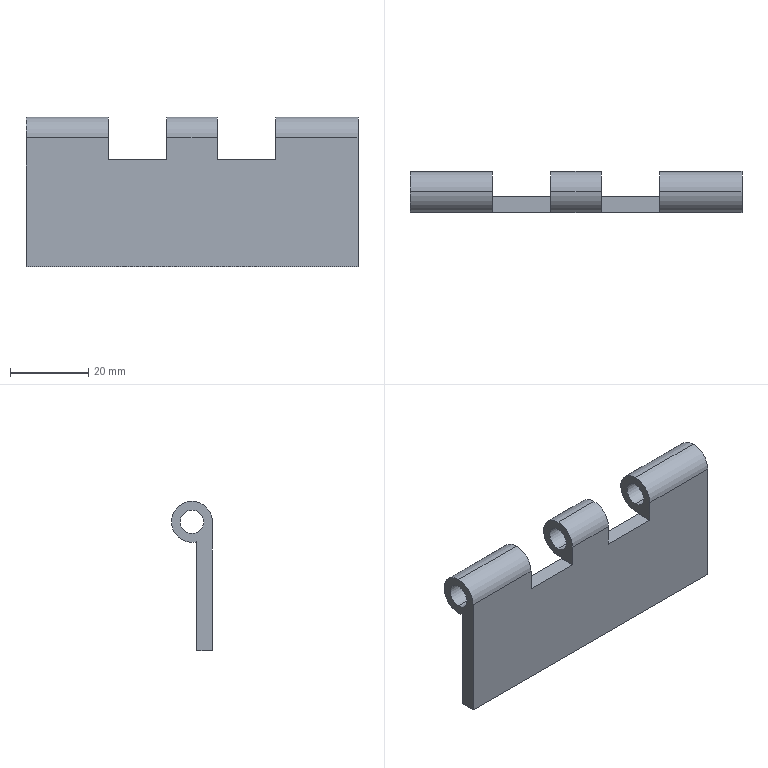Part | SolidWorks | features ICE 2, Chamfer 1, Cut 1, Extrusion 1 | 1 solid | 26 faces | box 85 x 10.5 x 38.25 mm | volume 12934 mm3 | cylinder 15 | plane 11 | commonest cylinder face diameters 10.5 x9 6 x6
STEP:
#1=CARTESIAN_POINT('',(21.5,0.,3.));
#2=VERTEX_POINT('',#1);
#3=CARTESIAN_POINT('',(21.5,0.,-3.));
#4=VERTEX_POINT('',#3);
#5=CARTESIAN_POINT('',(21.5,0.,0.));
#6=DIRECTION('',(1.,0.,0.));
#7=DIRECTION('',(0.,0.,-1.));
#8=AXIS2_PLACEMENT_3D('',#5,#6,#7);
#9=CIRCLE('',#8,3.);
#10=EDGE_CURVE('',#2,#4,#9,.T.);
#11=ORIENTED_EDGE('',*,*,#10,.F.);
#12=CARTESIAN_POINT('',(42.5,0.,3.));
#13=VERTEX_POINT('',#12);
#14=CARTESIAN_POINT('',(-42.5,0.,3.));
#15=DIRECTION('',(1.,0.,0.));
#16=VECTOR('',#15,1000.);
#17=LINE('',#14,#16);
#18=EDGE_CURVE('',#2,#13,#17,.T.);
#19=ORIENTED_EDGE('',*,*,#18,.T.);
#20=CARTESIAN_POINT('',(42.5,0.,-3.));
#21=VERTEX_POINT('',#20);
#22=CARTESIAN_POINT('',(42.5,0.,0.));
#23=DIRECTION('',(1.,0.,0.));
#24=DIRECTION('',(0.,0.,-1.));
#25=AXIS2_PLACEMENT_3D('',#22,#23,#24);
#26=CIRCLE('',#25,3.);
#27=EDGE_CURVE('',#13,#21,#26,.T.);
#28=ORIENTED_EDGE('',*,*,#27,.T.);
#29=CARTESIAN_POINT('',(-42.5,0.,-3.));
#30=DIRECTION('',(1.,0.,0.));
#31=VECTOR('',#30,1000.);
#32=LINE('',#29,#31);
#33=EDGE_CURVE('',#4,#21,#32,.T.);
#34=ORIENTED_EDGE('',*,*,#33,.F.);
#35=EDGE_LOOP('',(#11,#19,#28,#34));
#36=FACE_OUTER_BOUND('',#35,.T.);
#37=CARTESIAN_POINT('',(-42.5,0.,0.));
#38=DIRECTION('',(1.,0.,0.));
#39=DIRECTION('',(0.,0.,-1.));
#40=AXIS2_PLACEMENT_3D('',#37,#38,#39);
#41=CYLINDRICAL_SURFACE('',#40,3.);
#42=ADVANCED_FACE('',(#36),#41,.F.);
#43=CARTESIAN_POINT('',(-6.5,0.,3.));
#44=VERTEX_POINT('',#43);
#45=CARTESIAN_POINT('',(-6.5,0.,-3.));
#46=VERTEX_POINT('',#45);
#47=CARTESIAN_POINT('',(-6.5,0.,0.));
#48=DIRECTION('',(1.,0.,0.));
#49=DIRECTION('',(0.,0.,-1.));
#50=AXIS2_PLACEMENT_3D('',#47,#48,#49);
#51=CIRCLE('',#50,3.);
#52=EDGE_CURVE('',#44,#46,#51,.T.);
#53=ORIENTED_EDGE('',*,*,#52,.F.);
#54=CARTESIAN_POINT('',(6.5,0.,3.));
#55=VERTEX_POINT('',#54);
#56=CARTESIAN_POINT('',(-42.5,0.,3.));
#57=DIRECTION('',(1.,0.,0.));
#58=VECTOR('',#57,1000.);
#59=LINE('',#56,#58);
#60=EDGE_CURVE('',#44,#55,#59,.T.);
#61=ORIENTED_EDGE('',*,*,#60,.T.);
#62=CARTESIAN_POINT('',(6.5,0.,-3.));
#63=VERTEX_POINT('',#62);
#64=CARTESIAN_POINT('',(6.5,0.,0.));
#65=DIRECTION('',(-1.,0.,0.));
#66=DIRECTION('',(0.,0.,1.));
#67=AXIS2_PLACEMENT_3D('',#64,#65,#66);
#68=CIRCLE('',#67,3.);
#69=EDGE_CURVE('',#63,#55,#68,.T.);
#70=ORIENTED_EDGE('',*,*,#69,.F.);
#71=CARTESIAN_POINT('',(-42.5,0.,-3.));
#72=DIRECTION('',(1.,0.,0.));
#73=VECTOR('',#72,1000.);
#74=LINE('',#71,#73);
#75=EDGE_CURVE('',#46,#63,#74,.T.);
#76=ORIENTED_EDGE('',*,*,#75,.F.);
#77=EDGE_LOOP('',(#53,#61,#70,#76));
#78=FACE_OUTER_BOUND('',#77,.T.);
#79=CARTESIAN_POINT('',(-42.5,0.,0.));
#80=DIRECTION('',(1.,0.,0.));
#81=DIRECTION('',(0.,0.,-1.));
#82=AXIS2_PLACEMENT_3D('',#79,#80,#81);
#83=CYLINDRICAL_SURFACE('',#82,3.);
#84=ADVANCED_FACE('',(#78),#83,.F.);
#85=CARTESIAN_POINT('',(-42.5,0.,3.));
#86=VERTEX_POINT('',#85);
#87=CARTESIAN_POINT('',(-42.5,0.,-3.));
#88=VERTEX_POINT('',#87);
#89=CARTESIAN_POINT('',(-42.5,0.,0.));
#90=DIRECTION('',(1.,0.,0.));
#91=DIRECTION('',(0.,0.,-1.));
#92=AXIS2_PLACEMENT_3D('',#89,#90,#91);
#93=CIRCLE('',#92,3.);
#94=EDGE_CURVE('',#86,#88,#93,.T.);
#95=ORIENTED_EDGE('',*,*,#94,.F.);
#96=CARTESIAN_POINT('',(-21.5,0.,3.));
#97=VERTEX_POINT('',#96);
#98=CARTESIAN_POINT('',(-42.5,0.,3.));
#99=DIRECTION('',(1.,0.,0.));
#100=VECTOR('',#99,1000.);
#101=LINE('',#98,#100);
#102=EDGE_CURVE('',#86,#97,#101,.T.);
#103=ORIENTED_EDGE('',*,*,#102,.T.);
#104=CARTESIAN_POINT('',(-21.5,0.,-3.));
#105=VERTEX_POINT('',#104);
#106=CARTESIAN_POINT('',(-21.5,0.,0.));
#107=DIRECTION('',(-1.,0.,0.));
#108=DIRECTION('',(0.,0.,1.));
#109=AXIS2_PLACEMENT_3D('',#106,#107,#108);
#110=CIRCLE('',#109,3.);
#111=EDGE_CURVE('',#105,#97,#110,.T.);
#112=ORIENTED_EDGE('',*,*,#111,.F.);
#113=CARTESIAN_POINT('',(-42.5,0.,-3.));
#114=DIRECTION('',(1.,0.,0.));
#115=VECTOR('',#114,1000.);
#116=LINE('',#113,#115);
#117=EDGE_CURVE('',#88,#105,#116,.T.);
#118=ORIENTED_EDGE('',*,*,#117,.F.);
#119=EDGE_LOOP('',(#95,#103,#112,#118));
#120=FACE_OUTER_BOUND('',#119,.T.);
#121=CARTESIAN_POINT('',(-42.5,0.,0.));
#122=DIRECTION('',(1.,0.,0.));
#123=DIRECTION('',(0.,0.,-1.));
#124=AXIS2_PLACEMENT_3D('',#121,#122,#123);
#125=CYLINDRICAL_SURFACE('',#124,3.);
#126=ADVANCED_FACE('',(#120),#125,.F.);
#127=CARTESIAN_POINT('',(-21.5,0.,5.25));
#128=VERTEX_POINT('',#127);
#129=CARTESIAN_POINT('',(-21.5,0.,-5.25));
#130=VERTEX_POINT('',#129);
#131=CARTESIAN_POINT('',(-21.5,0.,0.));
#132=DIRECTION('',(-1.,0.,0.));
#133=DIRECTION('',(0.,0.,1.));
#134=AXIS2_PLACEMENT_3D('',#131,#132,#133);
#135=CIRCLE('',#134,5.25);
#136=EDGE_CURVE('',#128,#130,#135,.T.);
#137=ORIENTED_EDGE('',*,*,#136,.T.);
#138=CARTESIAN_POINT('',(-42.5,0.,-5.25));
#139=VERTEX_POINT('',#138);
#140=CARTESIAN_POINT('',(42.5,0.,-5.25));
#141=DIRECTION('',(-1.,0.,0.));
#142=VECTOR('',#141,1000.);
#143=LINE('',#140,#142);
#144=EDGE_CURVE('',#130,#139,#143,.T.);
#145=ORIENTED_EDGE('',*,*,#144,.T.);
#146=CARTESIAN_POINT('',(-42.5,0.,5.25));
#147=VERTEX_POINT('',#146);
#148=CARTESIAN_POINT('',(-42.5,0.,0.));
#149=DIRECTION('',(1.,0.,0.));
#150=DIRECTION('',(0.,0.,-1.));
#151=AXIS2_PLACEMENT_3D('',#148,#149,#150);
#152=CIRCLE('',#151,5.25);
#153=EDGE_CURVE('',#139,#147,#152,.T.);
#154=ORIENTED_EDGE('',*,*,#153,.T.);
#155=CARTESIAN_POINT('',(42.5,0.,5.25));
#156=DIRECTION('',(-1.,0.,0.));
#157=VECTOR('',#156,1000.);
#158=LINE('',#155,#157);
#159=EDGE_CURVE('',#128,#147,#158,.T.);
#160=ORIENTED_EDGE('',*,*,#159,.F.);
#161=EDGE_LOOP('',(#137,#145,#154,#160));
#162=FACE_OUTER_BOUND('',#161,.T.);
#163=CARTESIAN_POINT('',(42.5,0.,0.));
#164=DIRECTION('',(-1.,0.,0.));
#165=DIRECTION('',(0.,0.,1.));
#166=AXIS2_PLACEMENT_3D('',#163,#164,#165);
#167=CYLINDRICAL_SURFACE('',#166,5.25);
#168=ADVANCED_FACE('',(#162),#167,.T.);
#169=CARTESIAN_POINT('',(-21.5,-5.25,0.));
#170=VERTEX_POINT('',#169);
#171=CARTESIAN_POINT('',(-21.5,0.,0.));
#172=DIRECTION('',(-1.,0.,0.));
#173=DIRECTION('',(0.,0.,1.));
#174=AXIS2_PLACEMENT_3D('',#171,#172,#173);
#175=CIRCLE('',#174,5.25);
#176=EDGE_CURVE('',#170,#128,#175,.T.);
#177=ORIENTED_EDGE('',*,*,#176,.T.);
#178=ORIENTED_EDGE('',*,*,#159,.T.);
#179=CARTESIAN_POINT('',(-42.5,-5.25,0.));
#180=VERTEX_POINT('',#179);
#181=CARTESIAN_POINT('',(-42.5,0.,0.));
#182=DIRECTION('',(1.,0.,0.));
#183=DIRECTION('',(0.,0.,-1.));
#184=AXIS2_PLACEMENT_3D('',#181,#182,#183);
#185=CIRCLE('',#184,5.25);
#186=EDGE_CURVE('',#147,#180,#185,.T.);
#187=ORIENTED_EDGE('',*,*,#186,.T.);
#188=CARTESIAN_POINT('',(42.5,-5.25,0.));
#189=DIRECTION('',(-1.,0.,0.));
#190=VECTOR('',#189,1000.);
#191=LINE('',#188,#190);
#192=EDGE_CURVE('',#170,#180,#191,.T.);
#193=ORIENTED_EDGE('',*,*,#192,.F.);
#194=EDGE_LOOP('',(#177,#178,#187,#193));
#195=FACE_OUTER_BOUND('',#194,.T.);
#196=CARTESIAN_POINT('',(42.5,0.,0.));
#197=DIRECTION('',(-1.,0.,0.));
#198=DIRECTION('',(0.,0.,1.));
#199=AXIS2_PLACEMENT_3D('',#196,#197,#198);
#200=CYLINDRICAL_SURFACE('',#199,5.25);
#201=ADVANCED_FACE('',(#195),#200,.T.);
#202=CARTESIAN_POINT('',(42.5,0.,-5.25));
#203=VERTEX_POINT('',#202);
#204=CARTESIAN_POINT('',(42.5,0.,5.25));
#205=VERTEX_POINT('',#204);
#206=CARTESIAN_POINT('',(42.5,0.,0.));
#207=DIRECTION('',(1.,0.,0.));
#208=DIRECTION('',(0.,0.,-1.));
#209=AXIS2_PLACEMENT_3D('',#206,#207,#208);
#210=CIRCLE('',#209,5.25);
#211=EDGE_CURVE('',#203,#205,#210,.T.);
#212=ORIENTED_EDGE('',*,*,#211,.F.);
#213=CARTESIAN_POINT('',(21.5,0.,-5.25));
#214=VERTEX_POINT('',#213);
#215=CARTESIAN_POINT('',(42.5,0.,-5.25));
#216=DIRECTION('',(-1.,0.,0.));
#217=VECTOR('',#216,1000.);
#218=LINE('',#215,#217);
#219=EDGE_CURVE('',#203,#214,#218,.T.);
#220=ORIENTED_EDGE('',*,*,#219,.T.);
#221=CARTESIAN_POINT('',(21.5,0.,5.25));
#222=VERTEX_POINT('',#221);
#223=CARTESIAN_POINT('',(21.5,0.,0.));
#224=DIRECTION('',(1.,0.,0.));
#225=DIRECTION('',(0.,0.,-1.));
#226=AXIS2_PLACEMENT_3D('',#223,#224,#225);
#227=CIRCLE('',#226,5.25);
#228=EDGE_CURVE('',#214,#222,#227,.T.);
#229=ORIENTED_EDGE('',*,*,#228,.T.);
#230=CARTESIAN_POINT('',(42.5,0.,5.25));
#231=DIRECTION('',(-1.,0.,0.));
#232=VECTOR('',#231,1000.);
#233=LINE('',#230,#232);
#234=EDGE_CURVE('',#205,#222,#233,.T.);
#235=ORIENTED_EDGE('',*,*,#234,.F.);
#236=EDGE_LOOP('',(#212,#220,#229,#235));
#237=FACE_OUTER_BOUND('',#236,.T.);
#238=CARTESIAN_POINT('',(42.5,0.,0.));
#239=DIRECTION('',(-1.,0.,0.));
#240=DIRECTION('',(0.,0.,1.));
#241=AXIS2_PLACEMENT_3D('',#238,#239,#240);
#242=CYLINDRICAL_SURFACE('',#241,5.25);
#243=ADVANCED_FACE('',(#237),#242,.T.);
#244=CARTESIAN_POINT('',(42.5,-5.25,0.));
#245=VERTEX_POINT('',#244);
#246=CARTESIAN_POINT('',(42.5,0.,0.));
#247=DIRECTION('',(1.,0.,0.));
#248=DIRECTION('',(0.,0.,-1.));
#249=AXIS2_PLACEMENT_3D('',#246,#247,#248);
#250=CIRCLE('',#249,5.25);
#251=EDGE_CURVE('',#205,#245,#250,.T.);
#252=ORIENTED_EDGE('',*,*,#251,.F.);
#253=ORIENTED_EDGE('',*,*,#234,.T.);
#254=CARTESIAN_POINT('',(21.5,-5.25,0.));
#255=VERTEX_POINT('',#254);
#256=CARTESIAN_POINT('',(21.5,0.,0.));
#257=DIRECTION('',(1.,0.,0.));
#258=DIRECTION('',(0.,0.,-1.));
#259=AXIS2_PLACEMENT_3D('',#256,#257,#258);
#260=CIRCLE('',#259,5.25);
#261=EDGE_CURVE('',#222,#255,#260,.T.);
#262=ORIENTED_EDGE('',*,*,#261,.T.);
#263=CARTESIAN_POINT('',(42.5,-5.25,0.));
#264=DIRECTION('',(-1.,0.,0.));
#265=VECTOR('',#264,1000.);
#266=LINE('',#263,#265);
#267=EDGE_CURVE('',#245,#255,#266,.T.);
#268=ORIENTED_EDGE('',*,*,#267,.F.);
#269=EDGE_LOOP('',(#252,#253,#262,#268));
#270=FACE_OUTER_BOUND('',#269,.T.);
#271=CARTESIAN_POINT('',(42.5,0.,0.));
#272=DIRECTION('',(-1.,0.,0.));
#273=DIRECTION('',(0.,0.,1.));
#274=AXIS2_PLACEMENT_3D('',#271,#272,#273);
#275=CYLINDRICAL_SURFACE('',#274,5.25);
#276=ADVANCED_FACE('',(#270),#275,.T.);
#277=CARTESIAN_POINT('',(6.5,0.,5.25));
#278=VERTEX_POINT('',#277);
#279=CARTESIAN_POINT('',(6.5,0.,-5.25));
#280=VERTEX_POINT('',#279);
#281=CARTESIAN_POINT('',(6.5,0.,0.));
#282=DIRECTION('',(-1.,0.,0.));
#283=DIRECTION('',(0.,0.,1.));
#284=AXIS2_PLACEMENT_3D('',#281,#282,#283);
#285=CIRCLE('',#284,5.25);
#286=EDGE_CURVE('',#278,#280,#285,.T.);
#287=ORIENTED_EDGE('',*,*,#286,.T.);
#288=CARTESIAN_POINT('',(-6.5,0.,-5.25));
#289=VERTEX_POINT('',#288);
#290=CARTESIAN_POINT('',(42.5,0.,-5.25));
#291=DIRECTION('',(-1.,0.,0.));
#292=VECTOR('',#291,1000.);
#293=LINE('',#290,#292);
#294=EDGE_CURVE('',#280,#289,#293,.T.);
#295=ORIENTED_EDGE('',*,*,#294,.T.);
#296=CARTESIAN_POINT('',(-6.5,0.,5.25));
#297=VERTEX_POINT('',#296);
#298=CARTESIAN_POINT('',(-6.5,0.,0.));
#299=DIRECTION('',(1.,0.,0.));
#300=DIRECTION('',(0.,0.,-1.));
#301=AXIS2_PLACEMENT_3D('',#298,#299,#300);
#302=CIRCLE('',#301,5.25);
#303=EDGE_CURVE('',#289,#297,#302,.T.);
#304=ORIENTED_EDGE('',*,*,#303,.T.);
#305=CARTESIAN_POINT('',(42.5,0.,5.25));
#306=DIRECTION('',(-1.,0.,0.));
#307=VECTOR('',#306,1000.);
#308=LINE('',#305,#307);
#309=EDGE_CURVE('',#278,#297,#308,.T.);
#310=ORIENTED_EDGE('',*,*,#309,.F.);
#311=EDGE_LOOP('',(#287,#295,#304,#310));
#312=FACE_OUTER_BOUND('',#311,.T.);
#313=CARTESIAN_POINT('',(42.5,0.,0.));
#314=DIRECTION('',(-1.,0.,0.));
#315=DIRECTION('',(0.,0.,1.));
#316=AXIS2_PLACEMENT_3D('',#313,#314,#315);
#317=CYLINDRICAL_SURFACE('',#316,5.25);
#318=ADVANCED_FACE('',(#312),#317,.T.);
#319=CARTESIAN_POINT('',(6.5,-5.25,0.));
#320=VERTEX_POINT('',#319);
#321=CARTESIAN_POINT('',(6.5,0.,0.));
#322=DIRECTION('',(-1.,0.,0.));
#323=DIRECTION('',(0.,0.,1.));
#324=AXIS2_PLACEMENT_3D('',#321,#322,#323);
#325=CIRCLE('',#324,5.25);
#326=EDGE_CURVE('',#320,#278,#325,.T.);
#327=ORIENTED_EDGE('',*,*,#326,.T.);
#328=ORIENTED_EDGE('',*,*,#309,.T.);
#329=CARTESIAN_POINT('',(-6.5,-5.25,0.));
#330=VERTEX_POINT('',#329);
#331=CARTESIAN_POINT('',(-6.5,0.,0.));
#332=DIRECTION('',(1.,0.,0.));
#333=DIRECTION('',(0.,0.,-1.));
#334=AXIS2_PLACEMENT_3D('',#331,#332,#333);
#335=CIRCLE('',#334,5.25);
#336=EDGE_CURVE('',#297,#330,#335,.T.);
#337=ORIENTED_EDGE('',*,*,#336,.T.);
#338=CARTESIAN_POINT('',(42.5,-5.25,0.));
#339=DIRECTION('',(-1.,0.,0.));
#340=VECTOR('',#339,1000.);
#341=LINE('',#338,#340);
#342=EDGE_CURVE('',#320,#330,#341,.T.);
#343=ORIENTED_EDGE('',*,*,#342,.F.);
#344=EDGE_LOOP('',(#327,#328,#337,#343));
#345=FACE_OUTER_BOUND('',#344,.T.);
#346=CARTESIAN_POINT('',(42.5,0.,0.));
#347=DIRECTION('',(-1.,0.,0.));
#348=DIRECTION('',(0.,0.,1.));
#349=AXIS2_PLACEMENT_3D('',#346,#347,#348);
#350=CYLINDRICAL_SURFACE('',#349,5.25);
#351=ADVANCED_FACE('',(#345),#350,.T.);
#352=ORIENTED_EDGE('',*,*,#294,.F.);
#353=CARTESIAN_POINT('',(6.5,-1.25,-5.099));
#354=VERTEX_POINT('',#353);
#355=CARTESIAN_POINT('',(6.5,0.,0.));
#356=DIRECTION('',(-1.,0.,0.));
#357=DIRECTION('',(0.,0.,1.));
#358=AXIS2_PLACEMENT_3D('',#355,#356,#357);
#359=CIRCLE('',#358,5.25);
#360=EDGE_CURVE('',#280,#354,#359,.T.);
#361=ORIENTED_EDGE('',*,*,#360,.T.);
#362=CARTESIAN_POINT('',(-6.5,-1.25,-5.099));
#363=VERTEX_POINT('',#362);
#364=CARTESIAN_POINT('',(42.5,-1.25,-5.099));
#365=DIRECTION('',(-1.,0.,0.));
#366=VECTOR('',#365,1000.);
#367=LINE('',#364,#366);
#368=EDGE_CURVE('',#354,#363,#367,.T.);
#369=ORIENTED_EDGE('',*,*,#368,.T.);
#370=CARTESIAN_POINT('',(-6.5,0.,0.));
#371=DIRECTION('',(1.,0.,0.));
#372=DIRECTION('',(0.,0.,-1.));
#373=AXIS2_PLACEMENT_3D('',#370,#371,#372);
#374=CIRCLE('',#373,5.25);
#375=EDGE_CURVE('',#363,#289,#374,.T.);
#376=ORIENTED_EDGE('',*,*,#375,.T.);
#377=EDGE_LOOP('',(#352,#361,#369,#376));
#378=FACE_OUTER_BOUND('',#377,.T.);
#379=CARTESIAN_POINT('',(42.5,0.,0.));
#380=DIRECTION('',(-1.,0.,0.));
#381=DIRECTION('',(0.,0.,1.));
#382=AXIS2_PLACEMENT_3D('',#379,#380,#381);
#383=CYLINDRICAL_SURFACE('',#382,5.25);
#384=ADVANCED_FACE('',(#378),#383,.T.);
#385=ORIENTED_EDGE('',*,*,#219,.F.);
#386=CARTESIAN_POINT('',(42.5,-1.25,-5.099));
#387=VERTEX_POINT('',#386);
#388=CARTESIAN_POINT('',(42.5,0.,0.));
#389=DIRECTION('',(1.,0.,0.));
#390=DIRECTION('',(0.,0.,-1.));
#391=AXIS2_PLACEMENT_3D('',#388,#389,#390);
#392=CIRCLE('',#391,5.25);
#393=EDGE_CURVE('',#387,#203,#392,.T.);
#394=ORIENTED_EDGE('',*,*,#393,.F.);
#395=CARTESIAN_POINT('',(21.5,-1.25,-5.099));
#396=VERTEX_POINT('',#395);
#397=CARTESIAN_POINT('',(42.5,-1.25,-5.099));
#398=DIRECTION('',(-1.,0.,0.));
#399=VECTOR('',#398,1000.);
#400=LINE('',#397,#399);
#401=EDGE_CURVE('',#387,#396,#400,.T.);
#402=ORIENTED_EDGE('',*,*,#401,.T.);
#403=CARTESIAN_POINT('',(21.5,0.,0.));
#404=DIRECTION('',(1.,0.,0.));
#405=DIRECTION('',(0.,0.,-1.));
#406=AXIS2_PLACEMENT_3D('',#403,#404,#405);
#407=CIRCLE('',#406,5.25);
#408=EDGE_CURVE('',#396,#214,#407,.T.);
#409=ORIENTED_EDGE('',*,*,#408,.T.);
#410=EDGE_LOOP('',(#385,#394,#402,#409));
#411=FACE_OUTER_BOUND('',#410,.T.);
#412=CARTESIAN_POINT('',(42.5,0.,0.));
#413=DIRECTION('',(-1.,0.,0.));
#414=DIRECTION('',(0.,0.,1.));
#415=AXIS2_PLACEMENT_3D('',#412,#413,#414);
#416=CYLINDRICAL_SURFACE('',#415,5.25);
#417=ADVANCED_FACE('',(#411),#416,.T.);
#418=CARTESIAN_POINT('',(-42.5,-5.25,-33.));
#419=VERTEX_POINT('',#418);
#420=CARTESIAN_POINT('',(-42.5,-1.25,-33.));
#421=VERTEX_POINT('',#420);
#422=CARTESIAN_POINT('',(-42.5,-1.25,-33.));
#423=DIRECTION('',(0.,1.,0.));
#424=VECTOR('',#423,1000.);
#425=LINE('',#422,#424);
#426=EDGE_CURVE('',#419,#421,#425,.T.);
#427=ORIENTED_EDGE('',*,*,#426,.T.);
#428=CARTESIAN_POINT('',(42.5,-1.25,-33.));
#429=VERTEX_POINT('',#428);
#430=CARTESIAN_POINT('',(42.5,-1.25,-33.));
#431=DIRECTION('',(-1.,0.,0.));
#432=VECTOR('',#431,1000.);
#433=LINE('',#430,#432);
#434=EDGE_CURVE('',#429,#421,#433,.T.);
#435=ORIENTED_EDGE('',*,*,#434,.F.);
#436=CARTESIAN_POINT('',(42.5,-5.25,-33.));
#437=VERTEX_POINT('',#436);
#438=CARTESIAN_POINT('',(42.5,-1.25,-33.));
#439=DIRECTION('',(0.,1.,0.));
#440=VECTOR('',#439,1000.);
#441=LINE('',#438,#440);
#442=EDGE_CURVE('',#437,#429,#441,.T.);
#443=ORIENTED_EDGE('',*,*,#442,.F.);
#444=CARTESIAN_POINT('',(42.5,-5.25,-33.));
#445=DIRECTION('',(-1.,0.,0.));
#446=VECTOR('',#445,1000.);
#447=LINE('',#444,#446);
#448=EDGE_CURVE('',#437,#419,#447,.T.);
#449=ORIENTED_EDGE('',*,*,#448,.T.);
#450=EDGE_LOOP('',(#427,#435,#443,#449));
#451=FACE_OUTER_BOUND('',#450,.T.);
#452=CARTESIAN_POINT('',(42.5,-1.25,-33.));
#453=DIRECTION('',(0.,0.,1.));
#454=DIRECTION('',(1.,0.,0.));
#455=AXIS2_PLACEMENT_3D('',#452,#453,#454);
#456=PLANE('',#455);
#457=ADVANCED_FACE('',(#451),#456,.F.);
#458=CARTESIAN_POINT('',(-21.5,-1.25,-5.5));
#459=VERTEX_POINT('',#458);
#460=CARTESIAN_POINT('',(-6.5,-1.25,-5.5));
#461=VERTEX_POINT('',#460);
#462=CARTESIAN_POINT('',(42.5,-1.25,-5.5));
#463=DIRECTION('',(1.,0.,0.));
#464=VECTOR('',#463,1000.);
#465=LINE('',#462,#464);
#466=EDGE_CURVE('',#459,#461,#465,.T.);
#467=ORIENTED_EDGE('',*,*,#466,.T.);
#468=CARTESIAN_POINT('',(-6.5,-1.25,-5.099));
#469=DIRECTION('',(0.,0.,1.));
#470=VECTOR('',#469,1000.);
#471=LINE('',#468,#470);
#472=EDGE_CURVE('',#461,#363,#471,.T.);
#473=ORIENTED_EDGE('',*,*,#472,.T.);
#474=ORIENTED_EDGE('',*,*,#368,.F.);
#475=CARTESIAN_POINT('',(6.5,-1.25,-5.5));
#476=VERTEX_POINT('',#475);
#477=CARTESIAN_POINT('',(6.5,-1.25,-5.099));
#478=DIRECTION('',(0.,0.,-1.));
#479=VECTOR('',#478,1000.);
#480=LINE('',#477,#479);
#481=EDGE_CURVE('',#354,#476,#480,.T.);
#482=ORIENTED_EDGE('',*,*,#481,.T.);
#483=CARTESIAN_POINT('',(21.5,-1.25,-5.5));
#484=VERTEX_POINT('',#483);
#485=CARTESIAN_POINT('',(42.5,-1.25,-5.5));
#486=DIRECTION('',(1.,0.,0.));
#487=VECTOR('',#486,1000.);
#488=LINE('',#485,#487);
#489=EDGE_CURVE('',#476,#484,#488,.T.);
#490=ORIENTED_EDGE('',*,*,#489,.T.);
#491=CARTESIAN_POINT('',(21.5,-1.25,-5.099));
#492=DIRECTION('',(0.,0.,1.));
#493=VECTOR('',#492,1000.);
#494=LINE('',#491,#493);
#495=EDGE_CURVE('',#484,#396,#494,.T.);
#496=ORIENTED_EDGE('',*,*,#495,.T.);
#497=ORIENTED_EDGE('',*,*,#401,.F.);
#498=CARTESIAN_POINT('',(42.5,-1.25,-5.099));
#499=DIRECTION('',(0.,0.,1.));
#500=VECTOR('',#499,1000.);
#501=LINE('',#498,#500);
#502=EDGE_CURVE('',#429,#387,#501,.T.);
#503=ORIENTED_EDGE('',*,*,#502,.F.);
#504=ORIENTED_EDGE('',*,*,#434,.T.);
#505=CARTESIAN_POINT('',(-42.5,-1.25,-5.099));
#506=VERTEX_POINT('',#505);
#507=CARTESIAN_POINT('',(-42.5,-1.25,-5.099));
#508=DIRECTION('',(0.,0.,1.));
#509=VECTOR('',#508,1000.);
#510=LINE('',#507,#509);
#511=EDGE_CURVE('',#421,#506,#510,.T.);
#512=ORIENTED_EDGE('',*,*,#511,.T.);
#513=CARTESIAN_POINT('',(-21.5,-1.25,-5.099));
#514=VERTEX_POINT('',#513);
#515=CARTESIAN_POINT('',(42.5,-1.25,-5.099));
#516=DIRECTION('',(-1.,0.,0.));
#517=VECTOR('',#516,1000.);
#518=LINE('',#515,#517);
#519=EDGE_CURVE('',#514,#506,#518,.T.);
#520=ORIENTED_EDGE('',*,*,#519,.F.);
#521=CARTESIAN_POINT('',(-21.5,-1.25,-5.099));
#522=DIRECTION('',(0.,0.,-1.));
#523=VECTOR('',#522,1000.);
#524=LINE('',#521,#523);
#525=EDGE_CURVE('',#514,#459,#524,.T.);
#526=ORIENTED_EDGE('',*,*,#525,.T.);
#527=EDGE_LOOP('',(#467,#473,#474,#482,#490,#496,#497,#503,#504,#512,#520,#526));
#528=FACE_OUTER_BOUND('',#527,.T.);
#529=CARTESIAN_POINT('',(42.5,-1.25,-5.099));
#530=DIRECTION('',(0.,-1.,0.));
#531=DIRECTION('',(0.,0.,-1.));
#532=AXIS2_PLACEMENT_3D('',#529,#530,#531);
#533=PLANE('',#532);
#534=ADVANCED_FACE('',(#528),#533,.F.);
#535=ORIENTED_EDGE('',*,*,#144,.F.);
#536=CARTESIAN_POINT('',(-21.5,0.,0.));
#537=DIRECTION('',(-1.,0.,0.));
#538=DIRECTION('',(0.,0.,1.));
#539=AXIS2_PLACEMENT_3D('',#536,#537,#538);
#540=CIRCLE('',#539,5.25);
#541=EDGE_CURVE('',#130,#514,#540,.T.);
#542=ORIENTED_EDGE('',*,*,#541,.T.);
#543=ORIENTED_EDGE('',*,*,#519,.T.);
#544=CARTESIAN_POINT('',(-42.5,0.,0.));
#545=DIRECTION('',(1.,0.,0.));
#546=DIRECTION('',(0.,0.,-1.));
#547=AXIS2_PLACEMENT_3D('',#544,#545,#546);
#548=CIRCLE('',#547,5.25);
#549=EDGE_CURVE('',#506,#139,#548,.T.);
#550=ORIENTED_EDGE('',*,*,#549,.T.);
#551=EDGE_LOOP('',(#535,#542,#543,#550));
#552=FACE_OUTER_BOUND('',#551,.T.);
#553=CARTESIAN_POINT('',(42.5,0.,0.));
#554=DIRECTION('',(-1.,0.,0.));
#555=DIRECTION('',(0.,0.,1.));
#556=AXIS2_PLACEMENT_3D('',#553,#554,#555);
#557=CYLINDRICAL_SURFACE('',#556,5.25);
#558=ADVANCED_FACE('',(#552),#557,.T.);
#559=ORIENTED_EDGE('',*,*,#342,.T.);
#560=CARTESIAN_POINT('',(-6.5,-5.25,-5.5));
#561=VERTEX_POINT('',#560);
#562=CARTESIAN_POINT('',(-6.5,-5.25,0.));
#563=DIRECTION('',(0.,0.,-1.));
#564=VECTOR('',#563,1000.);
#565=LINE('',#562,#564);
#566=EDGE_CURVE('',#330,#561,#565,.T.);
#567=ORIENTED_EDGE('',*,*,#566,.T.);
#568=CARTESIAN_POINT('',(-21.5,-5.25,-5.5));
#569=VERTEX_POINT('',#568);
#570=CARTESIAN_POINT('',(42.5,-5.25,-5.5));
#571=DIRECTION('',(-1.,0.,0.));
#572=VECTOR('',#571,1000.);
#573=LINE('',#570,#572);
#574=EDGE_CURVE('',#561,#569,#573,.T.);
#575=ORIENTED_EDGE('',*,*,#574,.T.);
#576=CARTESIAN_POINT('',(-21.5,-5.25,0.));
#577=DIRECTION('',(0.,0.,1.));
#578=VECTOR('',#577,1000.);
#579=LINE('',#576,#578);
#580=EDGE_CURVE('',#569,#170,#579,.T.);
#581=ORIENTED_EDGE('',*,*,#580,.T.);
#582=ORIENTED_EDGE('',*,*,#192,.T.);
#583=CARTESIAN_POINT('',(-42.5,-5.25,0.));
#584=DIRECTION('',(0.,0.,-1.));
#585=VECTOR('',#584,1000.);
#586=LINE('',#583,#585);
#587=EDGE_CURVE('',#180,#419,#586,.T.);
#588=ORIENTED_EDGE('',*,*,#587,.T.);
#589=ORIENTED_EDGE('',*,*,#448,.F.);
#590=CARTESIAN_POINT('',(42.5,-5.25,0.));
#591=DIRECTION('',(0.,0.,-1.));
#592=VECTOR('',#591,1000.);
#593=LINE('',#590,#592);
#594=EDGE_CURVE('',#245,#437,#593,.T.);
#595=ORIENTED_EDGE('',*,*,#594,.F.);
#596=ORIENTED_EDGE('',*,*,#267,.T.);
#597=CARTESIAN_POINT('',(21.5,-5.25,-5.5));
#598=VERTEX_POINT('',#597);
#599=CARTESIAN_POINT('',(21.5,-5.25,0.));
#600=DIRECTION('',(0.,0.,-1.));
#601=VECTOR('',#600,1000.);
#602=LINE('',#599,#601);
#603=EDGE_CURVE('',#255,#598,#602,.T.);
#604=ORIENTED_EDGE('',*,*,#603,.T.);
#605=CARTESIAN_POINT('',(6.5,-5.25,-5.5));
#606=VERTEX_POINT('',#605);
#607=CARTESIAN_POINT('',(42.5,-5.25,-5.5));
#608=DIRECTION('',(-1.,0.,0.));
#609=VECTOR('',#608,1000.);
#610=LINE('',#607,#609);
#611=EDGE_CURVE('',#598,#606,#610,.T.);
#612=ORIENTED_EDGE('',*,*,#611,.T.);
#613=CARTESIAN_POINT('',(6.5,-5.25,0.));
#614=DIRECTION('',(0.,0.,1.));
#615=VECTOR('',#614,1000.);
#616=LINE('',#613,#615);
#617=EDGE_CURVE('',#606,#320,#616,.T.);
#618=ORIENTED_EDGE('',*,*,#617,.T.);
#619=EDGE_LOOP('',(#559,#567,#575,#581,#582,#588,#589,#595,#596,#604,#612,#618));
#620=FACE_OUTER_BOUND('',#619,.T.);
#621=CARTESIAN_POINT('',(42.5,-5.25,0.));
#622=DIRECTION('',(0.,1.,0.));
#623=DIRECTION('',(0.,0.,1.));
#624=AXIS2_PLACEMENT_3D('',#621,#622,#623);
#625=PLANE('',#624);
#626=ADVANCED_FACE('',(#620),#625,.F.);
#627=CARTESIAN_POINT('',(42.5,0.,0.));
#628=DIRECTION('',(1.,0.,0.));
#629=DIRECTION('',(0.,0.,-1.));
#630=AXIS2_PLACEMENT_3D('',#627,#628,#629);
#631=CIRCLE('',#630,3.);
#632=EDGE_CURVE('',#21,#13,#631,.T.);
#633=ORIENTED_EDGE('',*,*,#632,.F.);
#634=ORIENTED_EDGE('',*,*,#27,.F.);
#635=EDGE_LOOP('',(#633,#634));
#636=FACE_BOUND('',#635,.T.);
#637=ORIENTED_EDGE('',*,*,#442,.T.);
#638=ORIENTED_EDGE('',*,*,#502,.T.);
#639=ORIENTED_EDGE('',*,*,#393,.T.);
#640=ORIENTED_EDGE('',*,*,#211,.T.);
#641=ORIENTED_EDGE('',*,*,#251,.T.);
#642=ORIENTED_EDGE('',*,*,#594,.T.);
#643=EDGE_LOOP('',(#637,#638,#639,#640,#641,#642));
#644=FACE_OUTER_BOUND('',#643,.T.);
#645=CARTESIAN_POINT('',(42.5,0.,0.));
#646=DIRECTION('',(1.,0.,0.));
#647=DIRECTION('',(0.,0.,-1.));
#648=AXIS2_PLACEMENT_3D('',#645,#646,#647);
#649=PLANE('',#648);
#650=ADVANCED_FACE('',(#636,#644),#649,.T.);
#651=CARTESIAN_POINT('',(-42.5,0.,0.));
#652=DIRECTION('',(1.,0.,0.));
#653=DIRECTION('',(0.,0.,-1.));
#654=AXIS2_PLACEMENT_3D('',#651,#652,#653);
#655=CIRCLE('',#654,3.);
#656=EDGE_CURVE('',#88,#86,#655,.T.);
#657=ORIENTED_EDGE('',*,*,#656,.T.);
#658=ORIENTED_EDGE('',*,*,#94,.T.);
#659=EDGE_LOOP('',(#657,#658));
#660=FACE_BOUND('',#659,.T.);
#661=ORIENTED_EDGE('',*,*,#426,.F.);
#662=ORIENTED_EDGE('',*,*,#587,.F.);
#663=ORIENTED_EDGE('',*,*,#186,.F.);
#664=ORIENTED_EDGE('',*,*,#153,.F.);
#665=ORIENTED_EDGE('',*,*,#549,.F.);
#666=ORIENTED_EDGE('',*,*,#511,.F.);
#667=EDGE_LOOP('',(#661,#662,#663,#664,#665,#666));
#668=FACE_OUTER_BOUND('',#667,.T.);
#669=CARTESIAN_POINT('',(-42.5,0.,0.));
#670=DIRECTION('',(1.,0.,0.));
#671=DIRECTION('',(0.,0.,-1.));
#672=AXIS2_PLACEMENT_3D('',#669,#670,#671);
#673=PLANE('',#672);
#674=ADVANCED_FACE('',(#660,#668),#673,.F.);
#675=CARTESIAN_POINT('',(21.5,0.,0.));
#676=DIRECTION('',(1.,0.,0.));
#677=DIRECTION('',(0.,0.,-1.));
#678=AXIS2_PLACEMENT_3D('',#675,#676,#677);
#679=CIRCLE('',#678,3.);
#680=EDGE_CURVE('',#4,#2,#679,.T.);
#681=ORIENTED_EDGE('',*,*,#680,.T.);
#682=ORIENTED_EDGE('',*,*,#10,.T.);
#683=EDGE_LOOP('',(#681,#682));
#684=FACE_BOUND('',#683,.T.);
#685=CARTESIAN_POINT('',(21.5,-10.,-5.5));
#686=DIRECTION('',(0.,1.,0.));
#687=VECTOR('',#686,1000.);
#688=LINE('',#685,#687);
#689=EDGE_CURVE('',#598,#484,#688,.T.);
#690=ORIENTED_EDGE('',*,*,#689,.F.);
#691=ORIENTED_EDGE('',*,*,#603,.F.);
#692=ORIENTED_EDGE('',*,*,#261,.F.);
#693=ORIENTED_EDGE('',*,*,#228,.F.);
#694=ORIENTED_EDGE('',*,*,#408,.F.);
#695=ORIENTED_EDGE('',*,*,#495,.F.);
#696=EDGE_LOOP('',(#690,#691,#692,#693,#694,#695));
#697=FACE_OUTER_BOUND('',#696,.T.);
#698=CARTESIAN_POINT('',(21.5,-10.,5.5));
#699=DIRECTION('',(1.,0.,0.));
#700=DIRECTION('',(0.,0.,-1.));
#701=AXIS2_PLACEMENT_3D('',#698,#699,#700);
#702=PLANE('',#701);
#703=ADVANCED_FACE('',(#684,#697),#702,.F.);
#704=ORIENTED_EDGE('',*,*,#69,.T.);
#705=CARTESIAN_POINT('',(6.5,0.,0.));
#706=DIRECTION('',(-1.,0.,0.));
#707=DIRECTION('',(0.,0.,1.));
#708=AXIS2_PLACEMENT_3D('',#705,#706,#707);
#709=CIRCLE('',#708,3.);
#710=EDGE_CURVE('',#55,#63,#709,.T.);
#711=ORIENTED_EDGE('',*,*,#710,.T.);
#712=EDGE_LOOP('',(#704,#711));
#713=FACE_BOUND('',#712,.T.);
#714=ORIENTED_EDGE('',*,*,#326,.F.);
#715=ORIENTED_EDGE('',*,*,#617,.F.);
#716=CARTESIAN_POINT('',(6.5,-10.,-5.5));
#717=DIRECTION('',(0.,1.,0.));
#718=VECTOR('',#717,1000.);
#719=LINE('',#716,#718);
#720=EDGE_CURVE('',#606,#476,#719,.T.);
#721=ORIENTED_EDGE('',*,*,#720,.T.);
#722=ORIENTED_EDGE('',*,*,#481,.F.);
#723=ORIENTED_EDGE('',*,*,#360,.F.);
#724=ORIENTED_EDGE('',*,*,#286,.F.);
#725=EDGE_LOOP('',(#714,#715,#721,#722,#723,#724));
#726=FACE_OUTER_BOUND('',#725,.T.);
#727=CARTESIAN_POINT('',(6.5,-10.,5.5));
#728=DIRECTION('',(-1.,0.,0.));
#729=DIRECTION('',(0.,0.,1.));
#730=AXIS2_PLACEMENT_3D('',#727,#728,#729);
#731=PLANE('',#730);
#732=ADVANCED_FACE('',(#713,#726),#731,.F.);
#733=ORIENTED_EDGE('',*,*,#720,.F.);
#734=ORIENTED_EDGE('',*,*,#611,.F.);
#735=ORIENTED_EDGE('',*,*,#689,.T.);
#736=ORIENTED_EDGE('',*,*,#489,.F.);
#737=EDGE_LOOP('',(#733,#734,#735,#736));
#738=FACE_OUTER_BOUND('',#737,.T.);
#739=CARTESIAN_POINT('',(6.5,-10.,-5.5));
#740=DIRECTION('',(0.,0.,-1.));
#741=DIRECTION('',(-1.,0.,0.));
#742=AXIS2_PLACEMENT_3D('',#739,#740,#741);
#743=PLANE('',#742);
#744=ADVANCED_FACE('',(#738),#743,.F.);
#745=CARTESIAN_POINT('',(-6.5,0.,0.));
#746=DIRECTION('',(1.,0.,0.));
#747=DIRECTION('',(0.,0.,-1.));
#748=AXIS2_PLACEMENT_3D('',#745,#746,#747);
#749=CIRCLE('',#748,3.);
#750=EDGE_CURVE('',#46,#44,#749,.T.);
#751=ORIENTED_EDGE('',*,*,#750,.T.);
#752=ORIENTED_EDGE('',*,*,#52,.T.);
#753=EDGE_LOOP('',(#751,#752));
#754=FACE_BOUND('',#753,.T.);
#755=CARTESIAN_POINT('',(-6.5,-10.,-5.5));
#756=DIRECTION('',(0.,1.,0.));
#757=VECTOR('',#756,1000.);
#758=LINE('',#755,#757);
#759=EDGE_CURVE('',#561,#461,#758,.T.);
#760=ORIENTED_EDGE('',*,*,#759,.F.);
#761=ORIENTED_EDGE('',*,*,#566,.F.);
#762=ORIENTED_EDGE('',*,*,#336,.F.);
#763=ORIENTED_EDGE('',*,*,#303,.F.);
#764=ORIENTED_EDGE('',*,*,#375,.F.);
#765=ORIENTED_EDGE('',*,*,#472,.F.);
#766=EDGE_LOOP('',(#760,#761,#762,#763,#764,#765));
#767=FACE_OUTER_BOUND('',#766,.T.);
#768=CARTESIAN_POINT('',(-6.5,-10.,5.5));
#769=DIRECTION('',(1.,0.,0.));
#770=DIRECTION('',(0.,0.,-1.));
#771=AXIS2_PLACEMENT_3D('',#768,#769,#770);
#772=PLANE('',#771);
#773=ADVANCED_FACE('',(#754,#767),#772,.F.);
#774=ORIENTED_EDGE('',*,*,#111,.T.);
#775=CARTESIAN_POINT('',(-21.5,0.,0.));
#776=DIRECTION('',(-1.,0.,0.));
#777=DIRECTION('',(0.,0.,1.));
#778=AXIS2_PLACEMENT_3D('',#775,#776,#777);
#779=CIRCLE('',#778,3.);
#780=EDGE_CURVE('',#97,#105,#779,.T.);
#781=ORIENTED_EDGE('',*,*,#780,.T.);
#782=EDGE_LOOP('',(#774,#781));
#783=FACE_BOUND('',#782,.T.);
#784=ORIENTED_EDGE('',*,*,#176,.F.);
#785=ORIENTED_EDGE('',*,*,#580,.F.);
#786=CARTESIAN_POINT('',(-21.5,-10.,-5.5));
#787=DIRECTION('',(0.,1.,0.));
#788=VECTOR('',#787,1000.);
#789=LINE('',#786,#788);
#790=EDGE_CURVE('',#569,#459,#789,.T.);
#791=ORIENTED_EDGE('',*,*,#790,.T.);
#792=ORIENTED_EDGE('',*,*,#525,.F.);
#793=ORIENTED_EDGE('',*,*,#541,.F.);
#794=ORIENTED_EDGE('',*,*,#136,.F.);
#795=EDGE_LOOP('',(#784,#785,#791,#792,#793,#794));
#796=FACE_OUTER_BOUND('',#795,.T.);
#797=CARTESIAN_POINT('',(-21.5,-10.,5.5));
#798=DIRECTION('',(-1.,0.,0.));
#799=DIRECTION('',(0.,0.,1.));
#800=AXIS2_PLACEMENT_3D('',#797,#798,#799);
#801=PLANE('',#800);
#802=ADVANCED_FACE('',(#783,#796),#801,.F.);
#803=ORIENTED_EDGE('',*,*,#790,.F.);
#804=ORIENTED_EDGE('',*,*,#574,.F.);
#805=ORIENTED_EDGE('',*,*,#759,.T.);
#806=ORIENTED_EDGE('',*,*,#466,.F.);
#807=EDGE_LOOP('',(#803,#804,#805,#806));
#808=FACE_OUTER_BOUND('',#807,.T.);
#809=CARTESIAN_POINT('',(-6.5,-10.,-5.5));
#810=DIRECTION('',(0.,0.,-1.));
#811=DIRECTION('',(-1.,0.,0.));
#812=AXIS2_PLACEMENT_3D('',#809,#810,#811);
#813=PLANE('',#812);
#814=ADVANCED_FACE('',(#808),#813,.F.);
#815=ORIENTED_EDGE('',*,*,#102,.F.);
#816=ORIENTED_EDGE('',*,*,#656,.F.);
#817=ORIENTED_EDGE('',*,*,#117,.T.);
#818=ORIENTED_EDGE('',*,*,#780,.F.);
#819=EDGE_LOOP('',(#815,#816,#817,#818));
#820=FACE_OUTER_BOUND('',#819,.T.);
#821=CARTESIAN_POINT('',(-42.5,0.,0.));
#822=DIRECTION('',(1.,0.,0.));
#823=DIRECTION('',(0.,0.,-1.));
#824=AXIS2_PLACEMENT_3D('',#821,#822,#823);
#825=CYLINDRICAL_SURFACE('',#824,3.);
#826=ADVANCED_FACE('',(#820),#825,.F.);
#827=ORIENTED_EDGE('',*,*,#60,.F.);
#828=ORIENTED_EDGE('',*,*,#750,.F.);
#829=ORIENTED_EDGE('',*,*,#75,.T.);
#830=ORIENTED_EDGE('',*,*,#710,.F.);
#831=EDGE_LOOP('',(#827,#828,#829,#830));
#832=FACE_OUTER_BOUND('',#831,.T.);
#833=CARTESIAN_POINT('',(-42.5,0.,0.));
#834=DIRECTION('',(1.,0.,0.));
#835=DIRECTION('',(0.,0.,-1.));
#836=AXIS2_PLACEMENT_3D('',#833,#834,#835);
#837=CYLINDRICAL_SURFACE('',#836,3.);
#838=ADVANCED_FACE('',(#832),#837,.F.);
#839=ORIENTED_EDGE('',*,*,#18,.F.);
#840=ORIENTED_EDGE('',*,*,#680,.F.);
#841=ORIENTED_EDGE('',*,*,#33,.T.);
#842=ORIENTED_EDGE('',*,*,#632,.T.);
#843=EDGE_LOOP('',(#839,#840,#841,#842));
#844=FACE_OUTER_BOUND('',#843,.T.);
#845=CARTESIAN_POINT('',(-42.5,0.,0.));
#846=DIRECTION('',(1.,0.,0.));
#847=DIRECTION('',(0.,0.,-1.));
#848=AXIS2_PLACEMENT_3D('',#845,#846,#847);
#849=CYLINDRICAL_SURFACE('',#848,3.);
#850=ADVANCED_FACE('',(#844),#849,.F.);
#851=CLOSED_SHELL('',(#42,#84,#126,#168,#201,#243,#276,#318,#351,#384,#417,#457,#534,#558,#626,#650,#674,#703,#732,#744,#773,#802,#814,#826,#838,#850));
#852=MANIFOLD_SOLID_BREP('',#851);
#853=CARTESIAN_POINT('',(0.,0.,0.));
#854=DIRECTION('',(0.,0.,1.));
#855=DIRECTION('',(1.,0.,0.));
#856=AXIS2_PLACEMENT_3D('',#853,#854,#855);
#857=(LENGTH_UNIT()NAMED_UNIT(*)SI_UNIT(.MILLI.,.METRE.));
#858=UNCERTAINTY_MEASURE_WITH_UNIT(LENGTH_MEASURE(0.00001),#857,'','');
#859=(NAMED_UNIT(*)PLANE_ANGLE_UNIT()SI_UNIT($,.RADIAN.));
#860=(NAMED_UNIT(*)SI_UNIT($,.STERADIAN.)SOLID_ANGLE_UNIT());
#861=(GEOMETRIC_REPRESENTATION_CONTEXT(3)GLOBAL_UNCERTAINTY_ASSIGNED_CONTEXT((#858))GLOBAL_UNIT_ASSIGNED_CONTEXT((#857,#859,#860))REPRESENTATION_CONTEXT('',''));
#862=ADVANCED_BREP_SHAPE_REPRESENTATION('',(#852,#856),#861);